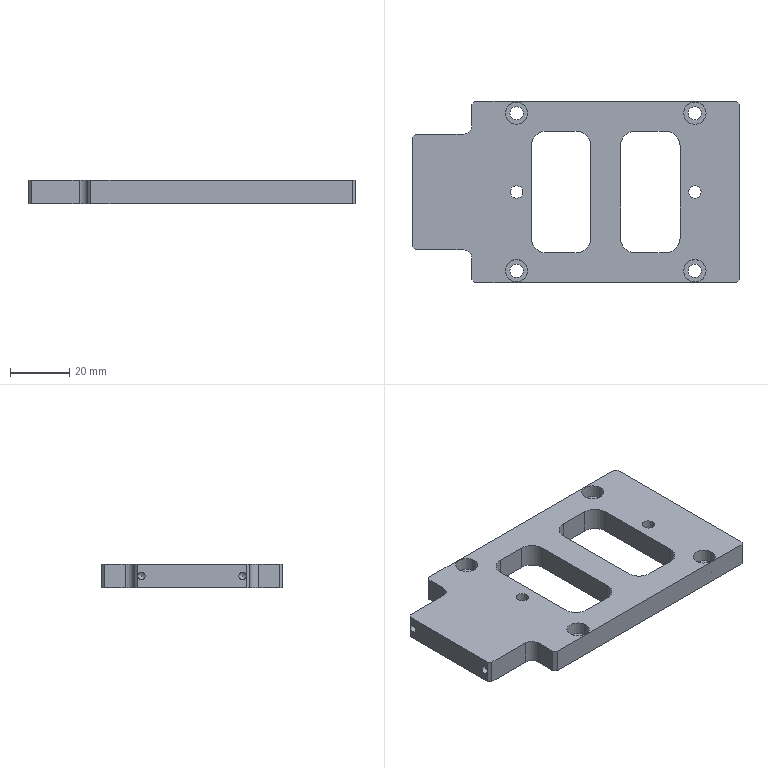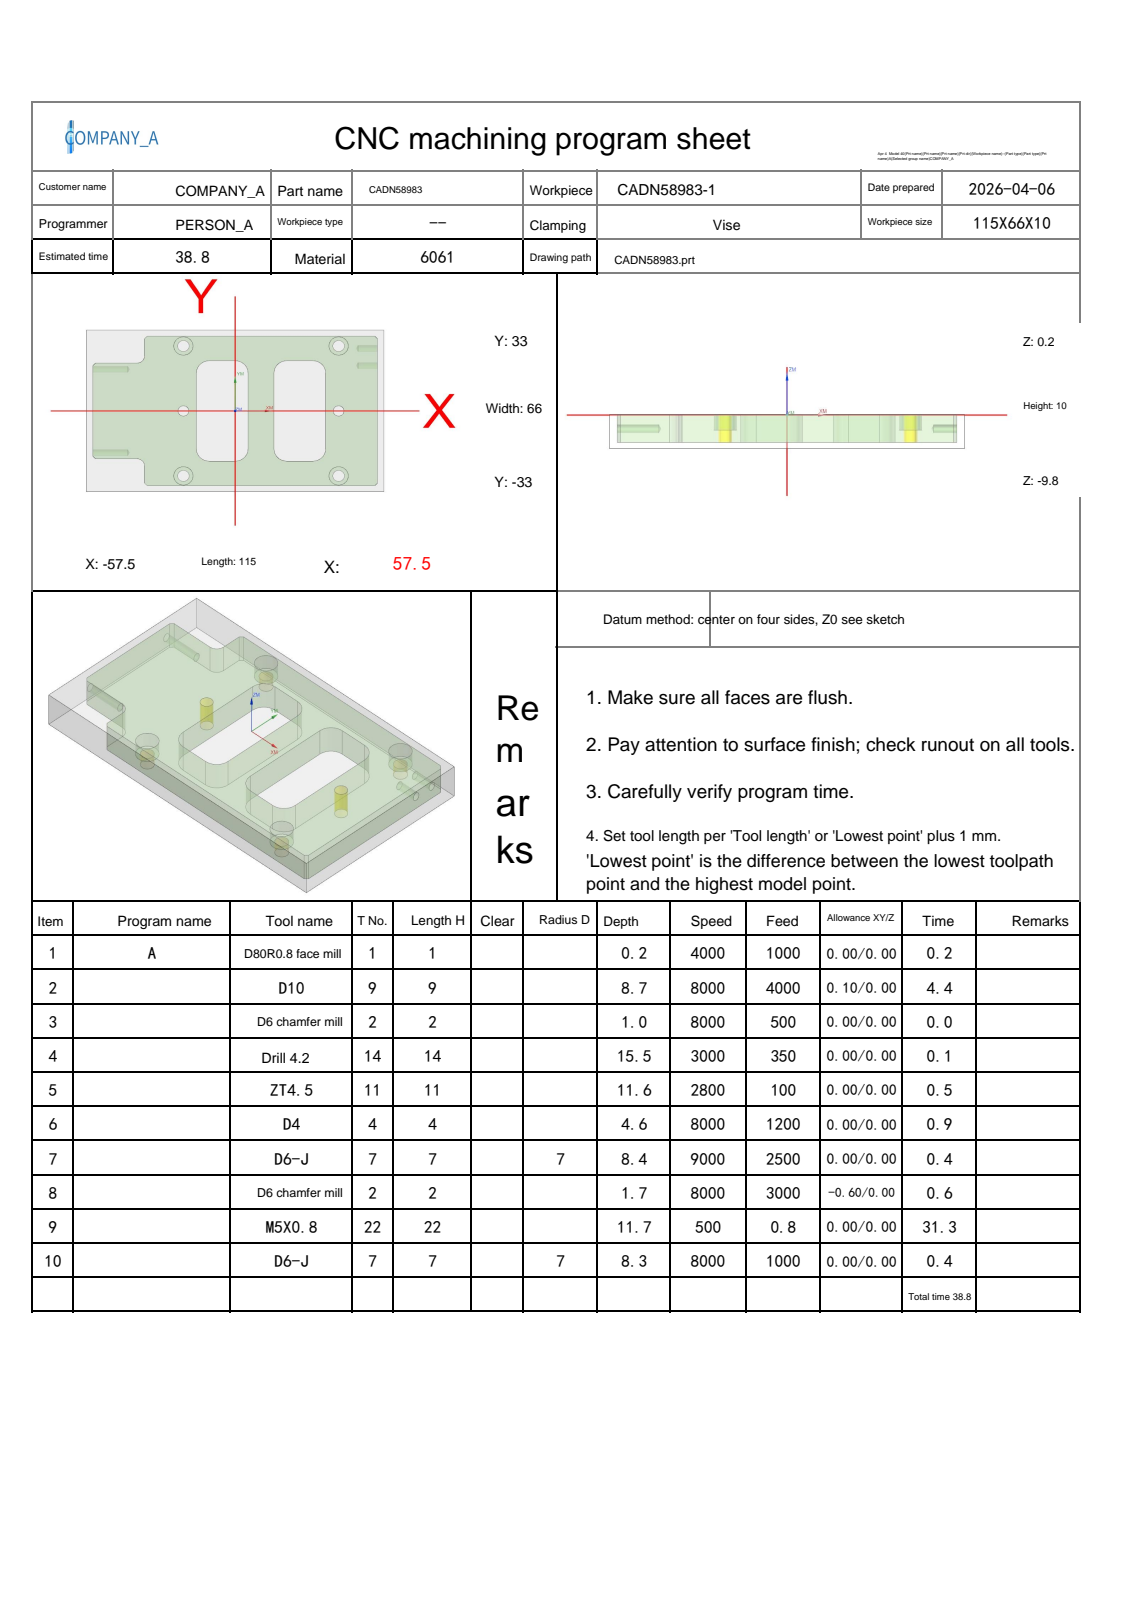NC program | NX | posted by the shop | part box 110 x 61 x 8 mm
Lines 1 to 34 of 4510:
%
O0001
(Machine time: 69.50 MIN)
(===Total Tool:8===)
(T1=D80R0.8 face mill D=80.  R=0.8  D-  H01 Z=0.    )
(T9=D10     D=10.  R=0.   D-  H09 Z=-8.5  )
(T2=D6 chamfer mill   D=6.   R=0.   D-  H02 Z=-1.5  )
(T14=Drill 4.2  D=4.2  DR_a=118 D-  H14 Z=-15.26)
(T11=ZT4.5  D=4.5  DR_a=118 D-  H11 Z=-11.35)
(T4=D4      D=4.   R=0.   D4  H04 Z=-4.4  )
(T7=D6-J    D=6.   R=0.   D7  H07 Z=-8.2  )
(T22=M5X0.8 D=4.2  DR_a=180 D-  H22 Z=-11.5 )
G80 G90 G17 G49 G40
G91 G28 Z0
M01
N1 T01 M06
(D80R0.8 face mill  D=80. R=0.8 H=01 ce=0.00 di=0.00)
G00 G90 G54 X-100. Y0.0 M03 S4000
G43 H01 Z20.
M08
Z2.
G01 Z0.0 F1000.
X-95.
X95.
X100.
Z2.
G00 Z20.
G91 G28 Z0.0
M05
M09
G91 G28 Z0.0
M01